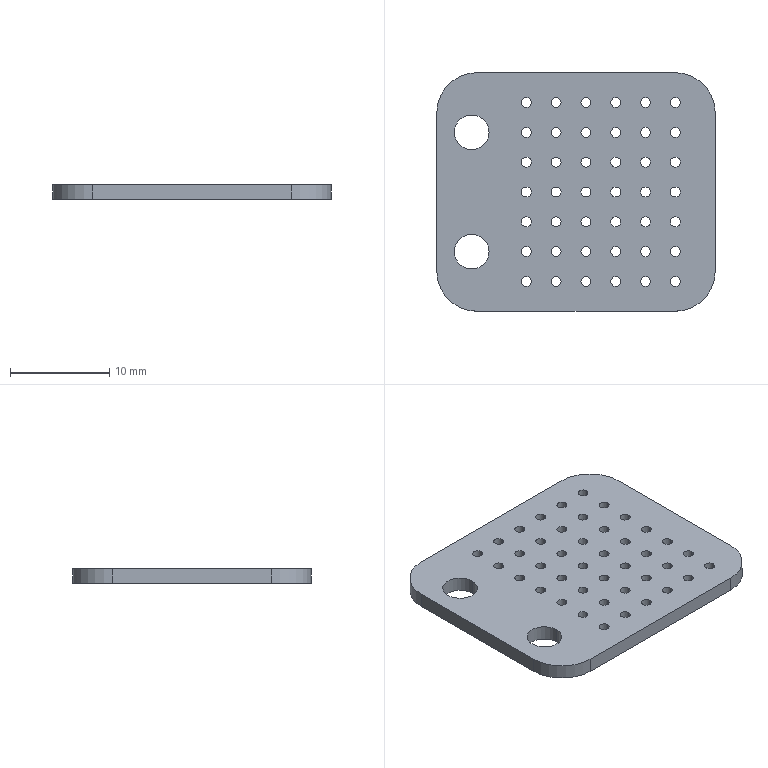Part | SolidWorks | features HoleWzd 2, Extrusion 1, Fillet 1, LPattern 1 | 1 solid | 98 faces | box 28 x 24 x 1.5 mm | volume 909.055 mm3 | cylinder 92 | plane 6 | commonest cylinder face diameters 1 x84 3.5 x4 8 x4